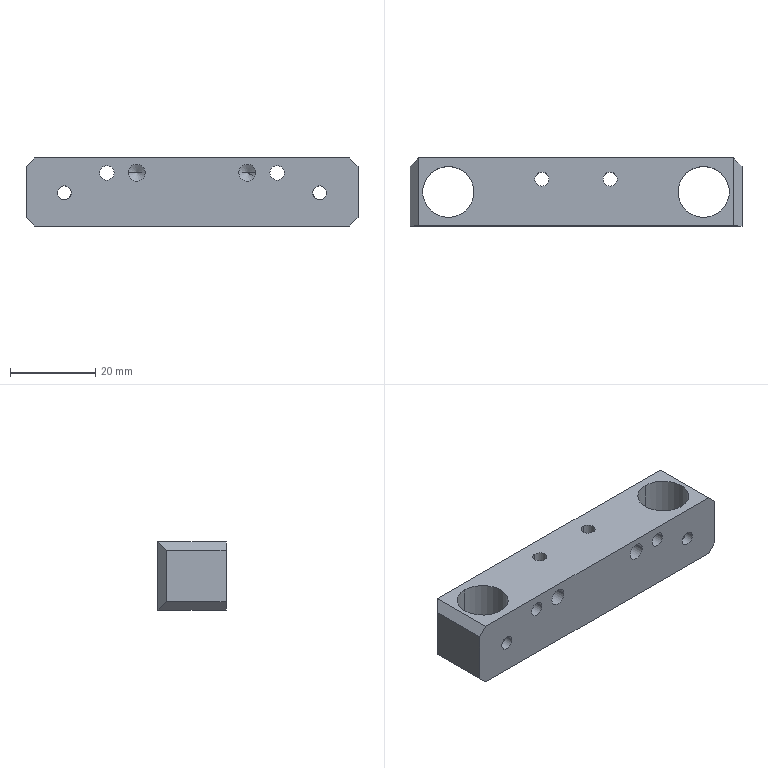NC program | NX | posted with a generic post | part box 78 x 16 x 16 mm
Lines 1 to 910 of 3743:
N10 G17 G21 G94 G90
(DRILLING , TOOL : ZXZ)
N12 T21 M6
N14 G54
N16 G17 G0 G90 X-30. Y0.2 B0. C0. S3500 M3
N18 G43 Z30. H21
N20 G94 G81 G98 Z-1. F250. R3.
N22 X-20. Y-4.5
N24 X-13.
N26 X13.
N28 X20.
N30 X30. Y0.2
N32 G80
N34 G0 X30. Y0.2 Z30.
N36 M5
(DRILLING_COPY_1 , TOOL : 3.4ZT)
N38 T24 M6
N40 G54
N42 G17 G0 G90 X-20. Y-4.5 B0. C0. S2000 M3
N44 G43 Z30. H24
N46 G94 G83 G98 Z-15.121 F150. Q2. R3.
N48 X-13. Z-11.021
N50 X13.
N52 X20. Z-15.121
N54 G80
N56 G0 X20. Y-4.5 Z30.
N58 M5
(DRILLING_COPY_1_COPY , TOOL : 3.3ZT)
N60 T13 M6
N62 G54
N64 G17 G0 G90 X-30. Y0.2 B0. C0. S2000 M3
N66 G43 Z30. H13
N68 G94 G83 G98 Z-17.991 F150. Q2. R3.
N70 X30.
N72 G80
N74 G0 X30. Y0.2 Z30.
N76 M5
(HOLE_MILLING_2 , TOOL : D2)
N78 T18 M6
N80 G54
N82 G17 G0 G90 X-13. Y-4.5 B0. C0. S7500 M3
N84 G43 Z30. H18
N86 Z0.5
N88 G94 G3 X-13.485 Y-4.015 R0.485 F800.
N90 X-13.97 Y-4.5 R0.485
N92 X-13.97 Y-4.5 Z0.475 I0.97 J0.
N94 X-13.97 Y-4.5 Z0.45 I0.97 J0.
N96 X-13.97 Y-4.5 Z0.425 I0.97 J0.
N98 X-13.97 Y-4.5 Z0.4 I0.97 J0.
N100 X-13.97 Y-4.5 Z0.375 I0.97 J0.
N102 X-13.97 Y-4.5 Z0.35 I0.97 J0.
N104 X-13.97 Y-4.5 Z0.325 I0.97 J0.
N106 X-13.97 Y-4.5 Z0.3 I0.97 J0.
N108 X-13.97 Y-4.5 Z0.275 I0.97 J0.
N110 X-13.97 Y-4.5 Z0.25 I0.97 J0.
N112 X-13.97 Y-4.5 Z0.225 I0.97 J0.
N114 X-13.97 Y-4.5 Z0.2 I0.97 J0.
N116 X-13.97 Y-4.5 Z0.175 I0.97 J0.
N118 X-13.97 Y-4.5 Z0.15 I0.97 J0.
N120 X-13.97 Y-4.5 Z0.125 I0.97 J0.
N122 X-13.97 Y-4.5 Z0.1 I0.97 J0.
N124 X-13.97 Y-4.5 Z0.075 I0.97 J0.
N126 X-13.97 Y-4.5 Z0.05 I0.97 J0.
N128 X-13.97 Y-4.5 Z0.025 I0.97 J0.
N130 X-13.97 Y-4.5 Z0. I0.97 J0.
N132 X-13.97 Y-4.5 Z-0.025 I0.97 J0.
N134 X-13.97 Y-4.5 Z-0.05 I0.97 J0.
N136 X-13.97 Y-4.5 Z-0.075 I0.97 J0.
N138 X-13.97 Y-4.5 Z-0.1 I0.97 J0.
N140 X-13.97 Y-4.5 Z-0.125 I0.97 J0.
N142 X-13.97 Y-4.5 Z-0.15 I0.97 J0.
N144 X-13.97 Y-4.5 Z-0.175 I0.97 J0.
N146 X-13.97 Y-4.5 Z-0.2 I0.97 J0.
N148 X-13.97 Y-4.5 Z-0.225 I0.97 J0.
N150 X-13.97 Y-4.5 Z-0.25 I0.97 J0.
N152 X-13.97 Y-4.5 Z-0.275 I0.97 J0.
N154 X-13.97 Y-4.5 Z-0.3 I0.97 J0.
N156 X-13.97 Y-4.5 Z-0.325 I0.97 J0.
N158 X-13.97 Y-4.5 Z-0.35 I0.97 J0.
N160 X-13.97 Y-4.5 Z-0.375 I0.97 J0.
N162 X-13.97 Y-4.5 Z-0.4 I0.97 J0.
N164 X-13.97 Y-4.5 Z-0.425 I0.97 J0.
N166 X-13.97 Y-4.5 Z-0.45 I0.97 J0.
N168 X-13.97 Y-4.5 Z-0.475 I0.97 J0.
N170 X-13.97 Y-4.5 Z-0.5 I0.97 J0.
N172 X-13.97 Y-4.5 Z-0.525 I0.97 J0.
N174 X-13.97 Y-4.5 Z-0.55 I0.97 J0.
N176 X-13.97 Y-4.5 Z-0.575 I0.97 J0.
N178 X-13.97 Y-4.5 Z-0.6 I0.97 J0.
N180 X-13.97 Y-4.5 Z-0.625 I0.97 J0.
N182 X-13.97 Y-4.5 Z-0.65 I0.97 J0.
N184 X-13.97 Y-4.5 Z-0.675 I0.97 J0.
N186 X-13.97 Y-4.5 Z-0.7 I0.97 J0.
N188 X-13.97 Y-4.5 Z-0.725 I0.97 J0.
N190 X-13.97 Y-4.5 Z-0.75 I0.97 J0.
N192 X-13.97 Y-4.5 Z-0.775 I0.97 J0.
N194 X-13.97 Y-4.5 Z-0.8 I0.97 J0.
N196 X-13.97 Y-4.5 Z-0.825 I0.97 J0.
N198 X-13.97 Y-4.5 Z-0.85 I0.97 J0.
N200 X-13.97 Y-4.5 Z-0.875 I0.97 J0.
N202 X-13.97 Y-4.5 Z-0.9 I0.97 J0.
N204 X-13.97 Y-4.5 Z-0.925 I0.97 J0.
N206 X-13.97 Y-4.5 Z-0.95 I0.97 J0.
N208 X-13.97 Y-4.5 Z-0.975 I0.97 J0.
N210 X-13.97 Y-4.5 Z-1. I0.97 J0.
N212 X-13.97 Y-4.5 Z-1.025 I0.97 J0.
N214 X-13.97 Y-4.5 Z-1.05 I0.97 J0.
N216 X-13.97 Y-4.5 Z-1.075 I0.97 J0.
N218 X-13.97 Y-4.5 Z-1.1 I0.97 J0.
N220 X-13.97 Y-4.5 Z-1.125 I0.97 J0.
N222 X-13.97 Y-4.5 Z-1.15 I0.97 J0.
N224 X-13.97 Y-4.5 Z-1.175 I0.97 J0.
N226 X-13.97 Y-4.5 Z-1.2 I0.97 J0.
N228 X-13.97 Y-4.5 Z-1.225 I0.97 J0.
N230 X-13.97 Y-4.5 Z-1.25 I0.97 J0.
N232 X-13.97 Y-4.5 Z-1.275 I0.97 J0.
N234 X-13.97 Y-4.5 Z-1.3 I0.97 J0.
N236 X-13.97 Y-4.5 Z-1.325 I0.97 J0.
N238 X-13.97 Y-4.5 Z-1.35 I0.97 J0.
N240 X-13.97 Y-4.5 Z-1.375 I0.97 J0.
N242 X-13.97 Y-4.5 Z-1.4 I0.97 J0.
N244 X-13.97 Y-4.5 Z-1.425 I0.97 J0.
N246 X-13.97 Y-4.5 Z-1.45 I0.97 J0.
N248 X-13.97 Y-4.5 Z-1.475 I0.97 J0.
N250 X-13.97 Y-4.5 Z-1.5 I0.97 J0.
N252 X-13.97 Y-4.5 Z-1.525 I0.97 J0.
N254 X-13.97 Y-4.5 Z-1.55 I0.97 J0.
N256 X-13.97 Y-4.5 Z-1.575 I0.97 J0.
N258 X-13.97 Y-4.5 Z-1.6 I0.97 J0.
N260 X-13.97 Y-4.5 Z-1.625 I0.97 J0.
N262 X-13.97 Y-4.5 Z-1.65 I0.97 J0.
N264 X-13.97 Y-4.5 Z-1.675 I0.97 J0.
N266 X-13.97 Y-4.5 Z-1.7 I0.97 J0.
N268 X-13.97 Y-4.5 Z-1.725 I0.97 J0.
N270 X-13.97 Y-4.5 Z-1.75 I0.97 J0.
N272 X-13.97 Y-4.5 Z-1.775 I0.97 J0.
N274 X-13.97 Y-4.5 Z-1.8 I0.97 J0.
N276 X-13.97 Y-4.5 Z-1.825 I0.97 J0.
N278 X-13.97 Y-4.5 Z-1.85 I0.97 J0.
N280 X-13.97 Y-4.5 Z-1.875 I0.97 J0.
N282 X-13.97 Y-4.5 Z-1.9 I0.97 J0.
N284 X-13.97 Y-4.5 Z-1.925 I0.97 J0.
N286 X-13.97 Y-4.5 Z-1.95 I0.97 J0.
N288 X-13.97 Y-4.5 Z-1.975 I0.97 J0.
N290 X-13.97 Y-4.5 Z-2. I0.97 J0.
N292 X-13.97 Y-4.5 Z-2.025 I0.97 J0.
N294 X-13.97 Y-4.5 Z-2.05 I0.97 J0.
N296 X-13.97 Y-4.5 Z-2.075 I0.97 J0.
N298 X-13.97 Y-4.5 Z-2.1 I0.97 J0.
N300 X-13.97 Y-4.5 Z-2.125 I0.97 J0.
N302 X-13.97 Y-4.5 Z-2.15 I0.97 J0.
N304 X-13.97 Y-4.5 Z-2.175 I0.97 J0.
N306 X-13.97 Y-4.5 Z-2.2 I0.97 J0.
N308 X-13.97 Y-4.5 Z-2.225 I0.97 J0.
N310 X-13.97 Y-4.5 Z-2.25 I0.97 J0.
N312 X-13.97 Y-4.5 Z-2.275 I0.97 J0.
N314 X-13.97 Y-4.5 Z-2.3 I0.97 J0.
N316 X-13.97 Y-4.5 Z-2.325 I0.97 J0.
N318 X-13.97 Y-4.5 Z-2.35 I0.97 J0.
N320 X-13.97 Y-4.5 Z-2.375 I0.97 J0.
N322 X-13.97 Y-4.5 Z-2.4 I0.97 J0.
N324 X-13.97 Y-4.5 Z-2.425 I0.97 J0.
N326 X-13.97 Y-4.5 Z-2.45 I0.97 J0.
N328 X-13.97 Y-4.5 Z-2.475 I0.97 J0.
N330 X-13.97 Y-4.5 Z-2.5 I0.97 J0.
N332 X-13.97 Y-4.5 Z-2.525 I0.97 J0.
N334 X-13.97 Y-4.5 Z-2.55 I0.97 J0.
N336 X-13.97 Y-4.5 Z-2.575 I0.97 J0.
N338 X-13.97 Y-4.5 Z-2.6 I0.97 J0.
N340 X-13.97 Y-4.5 Z-2.625 I0.97 J0.
N342 X-13.97 Y-4.5 Z-2.65 I0.97 J0.
N344 X-13.97 Y-4.5 Z-2.675 I0.97 J0.
N346 X-13.97 Y-4.5 Z-2.7 I0.97 J0.
N348 X-13.97 Y-4.5 Z-2.725 I0.97 J0.
N350 X-13.97 Y-4.5 Z-2.75 I0.97 J0.
N352 X-13.97 Y-4.5 Z-2.775 I0.97 J0.
N354 X-13.97 Y-4.5 Z-2.8 I0.97 J0.
N356 X-13.97 Y-4.5 Z-2.825 I0.97 J0.
N358 X-13.97 Y-4.5 Z-2.85 I0.97 J0.
N360 X-13.97 Y-4.5 Z-2.875 I0.97 J0.
N362 X-13.97 Y-4.5 Z-2.9 I0.97 J0.
N364 X-13.97 Y-4.5 Z-2.925 I0.97 J0.
N366 X-13.97 Y-4.5 Z-2.95 I0.97 J0.
N368 X-13.97 Y-4.5 Z-2.975 I0.97 J0.
N370 X-13.97 Y-4.5 Z-3. I0.97 J0.
N372 X-13.97 Y-4.5 Z-3.025 I0.97 J0.
N374 X-13.97 Y-4.5 Z-3.05 I0.97 J0.
N376 X-13.97 Y-4.5 Z-3.075 I0.97 J0.
N378 X-13.97 Y-4.5 Z-3.1 I0.97 J0.
N380 X-13.97 Y-4.5 Z-3.125 I0.97 J0.
N382 X-13.97 Y-4.5 Z-3.15 I0.97 J0.
N384 X-13.97 Y-4.5 Z-3.175 I0.97 J0.
N386 X-13.97 Y-4.5 Z-3.2 I0.97 J0.
N388 X-13.97 Y-4.5 Z-3.225 I0.97 J0.
N390 X-13.97 Y-4.5 Z-3.25 I0.97 J0.
N392 X-13.97 Y-4.5 Z-3.275 I0.97 J0.
N394 X-13.97 Y-4.5 Z-3.3 I0.97 J0.
N396 X-13.97 Y-4.5 Z-3.325 I0.97 J0.
N398 X-13.97 Y-4.5 Z-3.35 I0.97 J0.
N400 X-13.97 Y-4.5 Z-3.375 I0.97 J0.
N402 X-13.97 Y-4.5 Z-3.4 I0.97 J0.
N404 X-13.97 Y-4.5 Z-3.425 I0.97 J0.
N406 X-13.97 Y-4.5 Z-3.45 I0.97 J0.
N408 X-13.97 Y-4.5 Z-3.475 I0.97 J0.
N410 X-13.97 Y-4.5 Z-3.5 I0.97 J0.
N412 X-13.97 Y-4.5 Z-3.525 I0.97 J0.
N414 X-13.97 Y-4.5 Z-3.55 I0.97 J0.
N416 X-13.97 Y-4.5 Z-3.575 I0.97 J0.
N418 X-13.97 Y-4.5 Z-3.6 I0.97 J0.
N420 X-13.97 Y-4.5 Z-3.625 I0.97 J0.
N422 X-13.97 Y-4.5 Z-3.65 I0.97 J0.
N424 X-13.97 Y-4.5 Z-3.675 I0.97 J0.
N426 X-13.97 Y-4.5 Z-3.7 I0.97 J0.
N428 X-13.97 Y-4.5 Z-3.725 I0.97 J0.
N430 X-13.97 Y-4.5 Z-3.75 I0.97 J0.
N432 X-13.97 Y-4.5 Z-3.775 I0.97 J0.
N434 X-13.97 Y-4.5 Z-3.8 I0.97 J0.
N436 X-13.97 Y-4.5 Z-3.825 I0.97 J0.
N438 X-13.97 Y-4.5 Z-3.85 I0.97 J0.
N440 X-13.97 Y-4.5 Z-3.875 I0.97 J0.
N442 X-13.97 Y-4.5 Z-3.9 I0.97 J0.
N444 X-13.97 Y-4.5 Z-3.925 I0.97 J0.
N446 X-13.97 Y-4.5 Z-3.95 I0.97 J0.
N448 X-13.97 Y-4.5 Z-3.975 I0.97 J0.
N450 X-13.97 Y-4.5 Z-4. I0.97 J0.
N452 X-13.97 Y-4.5 Z-4.025 I0.97 J0.
N454 X-13.97 Y-4.5 Z-4.05 I0.97 J0.
N456 X-13.97 Y-4.5 Z-4.075 I0.97 J0.
N458 X-13.97 Y-4.5 Z-4.1 I0.97 J0.
N460 X-13.97 Y-4.5 Z-4.125 I0.97 J0.
N462 X-13.97 Y-4.5 Z-4.15 I0.97 J0.
N464 X-13.97 Y-4.5 Z-4.175 I0.97 J0.
N466 X-13.97 Y-4.5 Z-4.2 I0.97 J0.
N468 X-13.97 Y-4.5 Z-4.225 I0.97 J0.
N470 X-13.97 Y-4.5 Z-4.25 I0.97 J0.
N472 X-13.97 Y-4.5 Z-4.275 I0.97 J0.
N474 X-13.97 Y-4.5 Z-4.3 I0.97 J0.
N476 X-13.97 Y-4.5 Z-4.325 I0.97 J0.
N478 X-13.97 Y-4.5 Z-4.35 I0.97 J0.
N480 X-13.97 Y-4.5 Z-4.375 I0.97 J0.
N482 X-13.97 Y-4.5 Z-4.4 I0.97 J0.
N484 X-13.97 Y-4.5 Z-4.425 I0.97 J0.
N486 X-13.97 Y-4.5 Z-4.45 I0.97 J0.
N488 X-13.97 Y-4.5 Z-4.475 I0.97 J0.
N490 X-13.97 Y-4.5 Z-4.5 I0.97 J0.
N492 X-13.97 Y-4.5 Z-4.525 I0.97 J0.
N494 X-13.97 Y-4.5 Z-4.55 I0.97 J0.
N496 X-13.97 Y-4.5 Z-4.575 I0.97 J0.
N498 X-13.97 Y-4.5 Z-4.6 I0.97 J0.
N500 X-13.97 Y-4.5 Z-4.625 I0.97 J0.
N502 X-13.97 Y-4.5 Z-4.65 I0.97 J0.
N504 X-13.97 Y-4.5 Z-4.675 I0.97 J0.
N506 X-13.97 Y-4.5 Z-4.7 I0.97 J0.
N508 X-13.97 Y-4.5 Z-4.725 I0.97 J0.
N510 X-13.97 Y-4.5 Z-4.75 I0.97 J0.
N512 X-13.97 Y-4.5 Z-4.775 I0.97 J0.
N514 X-13.97 Y-4.5 Z-4.8 I0.97 J0.
N516 X-13.97 Y-4.5 Z-4.825 I0.97 J0.
N518 X-13.97 Y-4.5 Z-4.85 I0.97 J0.
N520 X-13.97 Y-4.5 Z-4.875 I0.97 J0.
N522 X-13.97 Y-4.5 Z-4.9 I0.97 J0.
N524 X-13.97 Y-4.5 Z-4.925 I0.97 J0.
N526 X-13.97 Y-4.5 Z-4.95 I0.97 J0.
N528 X-13.97 Y-4.5 Z-4.975 I0.97 J0.
N530 X-13.97 Y-4.5 Z-5. I0.97 J0.
N532 X-13.97 Y-4.5 Z-5.025 I0.97 J0.
N534 X-13.97 Y-4.5 Z-5.05 I0.97 J0.
N536 X-13.97 Y-4.5 Z-5.075 I0.97 J0.
N538 X-13.97 Y-4.5 Z-5.1 I0.97 J0.
N540 X-13.97 Y-4.5 Z-5.125 I0.97 J0.
N542 X-13.97 Y-4.5 Z-5.15 I0.97 J0.
N544 X-13.97 Y-4.5 Z-5.175 I0.97 J0.
N546 X-13.97 Y-4.5 Z-5.2 I0.97 J0.
N548 X-13.97 Y-4.5 Z-5.225 I0.97 J0.
N550 X-13.97 Y-4.5 Z-5.25 I0.97 J0.
N552 X-13.97 Y-4.5 Z-5.275 I0.97 J0.
N554 X-13.97 Y-4.5 Z-5.3 I0.97 J0.
N556 X-13.97 Y-4.5 Z-5.325 I0.97 J0.
N558 X-13.97 Y-4.5 Z-5.35 I0.97 J0.
N560 X-13.97 Y-4.5 Z-5.375 I0.97 J0.
N562 X-13.97 Y-4.5 Z-5.4 I0.97 J0.
N564 X-13.97 Y-4.5 Z-5.425 I0.97 J0.
N566 X-13.97 Y-4.5 Z-5.45 I0.97 J0.
N568 X-13.97 Y-4.5 Z-5.475 I0.97 J0.
N570 X-13.97 Y-4.5 Z-5.5 I0.97 J0.
N572 X-13.97 Y-4.5 Z-5.525 I0.97 J0.
N574 X-13.97 Y-4.5 Z-5.55 I0.97 J0.
N576 X-13.97 Y-4.5 Z-5.575 I0.97 J0.
N578 X-13.97 Y-4.5 Z-5.6 I0.97 J0.
N580 X-13.97 Y-4.5 Z-5.625 I0.97 J0.
N582 X-13.97 Y-4.5 Z-5.65 I0.97 J0.
N584 X-13.97 Y-4.5 Z-5.675 I0.97 J0.
N586 X-13.97 Y-4.5 Z-5.7 I0.97 J0.
N588 X-13.97 Y-4.5 Z-5.725 I0.97 J0.
N590 X-13.97 Y-4.5 Z-5.75 I0.97 J0.
N592 X-13.97 Y-4.5 Z-5.775 I0.97 J0.
N594 X-13.97 Y-4.5 Z-5.8 I0.97 J0.
N596 X-13.97 Y-4.5 Z-5.825 I0.97 J0.
N598 X-13.97 Y-4.5 Z-5.85 I0.97 J0.
N600 X-13.97 Y-4.5 Z-5.875 I0.97 J0.
N602 X-13.97 Y-4.5 Z-5.9 I0.97 J0.
N604 X-13.97 Y-4.5 Z-5.925 I0.97 J0.
N606 X-13.97 Y-4.5 Z-5.95 I0.97 J0.
N608 X-13.97 Y-4.5 Z-5.975 I0.97 J0.
N610 X-13.97 Y-4.5 Z-6. I0.97 J0.
N612 X-13.97 Y-4.5 Z-6.025 I0.97 J0.
N614 X-13.97 Y-4.5 Z-6.05 I0.97 J0.
N616 X-13.97 Y-4.5 Z-6.075 I0.97 J0.
N618 X-13.97 Y-4.5 Z-6.1 I0.97 J0.
N620 X-13.97 Y-4.5 Z-6.125 I0.97 J0.
N622 X-13.97 Y-4.5 Z-6.15 I0.97 J0.
N624 X-13.97 Y-4.5 Z-6.175 I0.97 J0.
N626 X-13.97 Y-4.5 Z-6.2 I0.97 J0.
N628 X-13.97 Y-4.5 Z-6.225 I0.97 J0.
N630 X-13.97 Y-4.5 Z-6.25 I0.97 J0.
N632 X-13.97 Y-4.5 Z-6.275 I0.97 J0.
N634 X-13.97 Y-4.5 Z-6.3 I0.97 J0.
N636 X-13.97 Y-4.5 Z-6.325 I0.97 J0.
N638 X-13.97 Y-4.5 Z-6.35 I0.97 J0.
N640 X-13.97 Y-4.5 Z-6.375 I0.97 J0.
N642 X-13.97 Y-4.5 Z-6.4 I0.97 J0.
N644 X-13.97 Y-4.5 Z-6.425 I0.97 J0.
N646 X-13.97 Y-4.5 Z-6.45 I0.97 J0.
N648 X-13.97 Y-4.5 Z-6.475 I0.97 J0.
N650 X-13.97 Y-4.5 Z-6.5 I0.97 J0.
N652 X-13.97 Y-4.5 Z-6.525 I0.97 J0.
N654 X-13.97 Y-4.5 Z-6.55 I0.97 J0.
N656 X-13.97 Y-4.5 Z-6.575 I0.97 J0.
N658 X-13.97 Y-4.5 Z-6.6 I0.97 J0.
N660 X-13.97 Y-4.5 Z-6.625 I0.97 J0.
N662 X-13.97 Y-4.5 Z-6.65 I0.97 J0.
N664 X-13.97 Y-4.5 Z-6.675 I0.97 J0.
N666 X-13.97 Y-4.5 Z-6.7 I0.97 J0.
N668 X-13.97 Y-4.5 Z-6.725 I0.97 J0.
N670 X-13.97 Y-4.5 Z-6.75 I0.97 J0.
N672 X-13.97 Y-4.5 Z-6.775 I0.97 J0.
N674 X-13.97 Y-4.5 Z-6.8 I0.97 J0.
N676 X-13.97 Y-4.5 Z-6.825 I0.97 J0.
N678 X-13.97 Y-4.5 Z-6.85 I0.97 J0.
N680 X-13.97 Y-4.5 Z-6.875 I0.97 J0.
N682 X-13.97 Y-4.5 Z-6.9 I0.97 J0.
N684 X-13.97 Y-4.5 Z-6.925 I0.97 J0.
N686 X-13.97 Y-4.5 Z-6.95 I0.97 J0.
N688 X-13.97 Y-4.5 Z-6.975 I0.97 J0.
N690 X-13.97 Y-4.5 Z-7. I0.97 J0.
N692 X-13.97 Y-4.5 Z-7.025 I0.97 J0.
N694 X-13.97 Y-4.5 Z-7.05 I0.97 J0.
N696 X-13.97 Y-4.5 Z-7.075 I0.97 J0.
N698 X-13.97 Y-4.5 Z-7.1 I0.97 J0.
N700 X-13.97 Y-4.5 Z-7.125 I0.97 J0.
N702 X-13.97 Y-4.5 Z-7.15 I0.97 J0.
N704 X-13.97 Y-4.5 Z-7.175 I0.97 J0.
N706 X-13.97 Y-4.5 Z-7.2 I0.97 J0.
N708 X-13.97 Y-4.5 Z-7.225 I0.97 J0.
N710 X-13.97 Y-4.5 Z-7.25 I0.97 J0.
N712 X-13.97 Y-4.5 Z-7.275 I0.97 J0.
N714 X-13.97 Y-4.5 Z-7.3 I0.97 J0.
N716 X-13.97 Y-4.5 Z-7.325 I0.97 J0.
N718 X-13.97 Y-4.5 Z-7.35 I0.97 J0.
N720 X-13.97 Y-4.5 Z-7.375 I0.97 J0.
N722 X-13.97 Y-4.5 Z-7.4 I0.97 J0.
N724 X-13.97 Y-4.5 Z-7.425 I0.97 J0.
N726 X-13.97 Y-4.5 Z-7.45 I0.97 J0.
N728 X-13.97 Y-4.5 Z-7.475 I0.97 J0.
N730 X-13.97 Y-4.5 Z-7.5 I0.97 J0.
N732 X-13.97 Y-4.5 Z-7.525 I0.97 J0.
N734 X-13.97 Y-4.5 Z-7.55 I0.97 J0.
N736 X-13.97 Y-4.5 Z-7.575 I0.97 J0.
N738 X-13.97 Y-4.5 Z-7.6 I0.97 J0.
N740 X-13.97 Y-4.5 Z-7.625 I0.97 J0.
N742 X-13.97 Y-4.5 Z-7.65 I0.97 J0.
N744 X-13.97 Y-4.5 Z-7.675 I0.97 J0.
N746 X-13.97 Y-4.5 Z-7.7 I0.97 J0.
N748 X-13.97 Y-4.5 Z-7.725 I0.97 J0.
N750 X-13.97 Y-4.5 Z-7.75 I0.97 J0.
N752 X-13.97 Y-4.5 Z-7.775 I0.97 J0.
N754 X-13.97 Y-4.5 Z-7.8 I0.97 J0.
N756 X-13.97 Y-4.5 Z-7.825 I0.97 J0.
N758 X-13.97 Y-4.5 Z-7.85 I0.97 J0.
N760 X-13.97 Y-4.5 Z-7.875 I0.97 J0.
N762 X-13.97 Y-4.5 Z-7.9 I0.97 J0.
N764 X-13.97 Y-4.5 Z-7.925 I0.97 J0.
N766 X-13.97 Y-4.5 Z-7.95 I0.97 J0.
N768 X-13.97 Y-4.5 Z-7.975 I0.97 J0.
N770 X-13.97 Y-4.5 Z-8. I0.97 J0.
N772 X-13.97 Y-4.5 Z-8.025 I0.97 J0.
N774 X-13.97 Y-4.5 Z-8.05 I0.97 J0.
N776 X-13.97 Y-4.5 Z-8.075 I0.97 J0.
N778 X-13.97 Y-4.5 Z-8.1 I0.97 J0.
N780 X-13.97 Y-4.5 Z-8.125 I0.97 J0.
N782 X-13.97 Y-4.5 Z-8.15 I0.97 J0.
N784 X-13.97 Y-4.5 Z-8.175 I0.97 J0.
N786 X-13.97 Y-4.5 Z-8.2 I0.97 J0.
N788 X-13.97 Y-4.5 Z-8.225 I0.97 J0.
N790 X-13.97 Y-4.5 Z-8.25 I0.97 J0.
N792 X-13.97 Y-4.5 Z-8.275 I0.97 J0.
N794 X-13.97 Y-4.5 Z-8.3 I0.97 J0.
N796 X-13.97 Y-4.5 Z-8.325 I0.97 J0.
N798 X-13.97 Y-4.5 Z-8.35 I0.97 J0.
N800 X-13.97 Y-4.5 Z-8.375 I0.97 J0.
N802 X-13.97 Y-4.5 Z-8.4 I0.97 J0.
N804 X-13.97 Y-4.5 Z-8.425 I0.97 J0.
N806 X-13.97 Y-4.5 Z-8.45 I0.97 J0.
N808 X-13.97 Y-4.5 Z-8.475 I0.97 J0.
N810 X-13.97 Y-4.5 Z-8.5 I0.97 J0.
N812 X-13.97 Y-4.5 Z-8.525 I0.97 J0.
N814 X-13.97 Y-4.5 Z-8.55 I0.97 J0.
N816 X-13.97 Y-4.5 Z-8.575 I0.97 J0.
N818 X-13.97 Y-4.5 Z-8.6 I0.97 J0.
N820 X-13.97 Y-4.5 Z-8.625 I0.97 J0.
N822 X-13.97 Y-4.5 Z-8.65 I0.97 J0.
N824 X-13.97 Y-4.5 Z-8.675 I0.97 J0.
N826 X-13.97 Y-4.5 Z-8.7 I0.97 J0.
N828 X-13.97 Y-4.5 Z-8.725 I0.97 J0.
N830 X-13.97 Y-4.5 Z-8.75 I0.97 J0.
N832 X-13.97 Y-4.5 Z-8.775 I0.97 J0.
N834 X-13.97 Y-4.5 Z-8.8 I0.97 J0.
N836 X-13.97 Y-4.5 Z-8.825 I0.97 J0.
N838 X-13.97 Y-4.5 Z-8.85 I0.97 J0.
N840 X-13.97 Y-4.5 Z-8.875 I0.97 J0.
N842 X-13.97 Y-4.5 Z-8.9 I0.97 J0.
N844 X-13.97 Y-4.5 Z-8.925 I0.97 J0.
N846 X-13.97 Y-4.5 Z-8.95 I0.97 J0.
N848 X-13.97 Y-4.5 Z-8.975 I0.97 J0.
N850 X-13.97 Y-4.5 Z-9. I0.97 J0.
N852 X-13.97 Y-4.5 Z-9.025 I0.97 J0.
N854 X-13.97 Y-4.5 Z-9.05 I0.97 J0.
N856 X-13.97 Y-4.5 Z-9.075 I0.97 J0.
N858 X-13.97 Y-4.5 Z-9.1 I0.97 J0.
N860 X-13.97 Y-4.5 Z-9.125 I0.97 J0.
N862 X-13.97 Y-4.5 Z-9.15 I0.97 J0.
N864 X-13.97 Y-4.5 Z-9.175 I0.97 J0.
N866 X-13.97 Y-4.5 Z-9.2 I0.97 J0.
N868 X-13.97 Y-4.5 Z-9.225 I0.97 J0.
N870 X-13.97 Y-4.5 Z-9.25 I0.97 J0.
N872 X-13.97 Y-4.5 Z-9.275 I0.97 J0.
N874 X-13.97 Y-4.5 Z-9.3 I0.97 J0.
N876 X-13.97 Y-4.5 Z-9.325 I0.97 J0.
N878 X-13.97 Y-4.5 Z-9.35 I0.97 J0.
N880 X-13.97 Y-4.5 Z-9.375 I0.97 J0.
N882 X-13.97 Y-4.5 Z-9.4 I0.97 J0.
N884 X-13.97 Y-4.5 Z-9.425 I0.97 J0.
N886 X-13.97 Y-4.5 Z-9.45 I0.97 J0.
N888 X-13.97 Y-4.5 Z-9.475 I0.97 J0.
N890 X-13.97 Y-4.5 Z-9.5 I0.97 J0.
N892 X-13.97 Y-4.5 Z-9.525 I0.97 J0.
N894 X-13.97 Y-4.5 Z-9.55 I0.97 J0.
N896 X-13.97 Y-4.5 Z-9.575 I0.97 J0.
N898 X-13.97 Y-4.5 Z-9.6 I0.97 J0.
N900 X-13.97 Y-4.5 Z-9.625 I0.97 J0.
N902 X-13.97 Y-4.5 Z-9.65 I0.97 J0.
N904 X-13.97 Y-4.5 Z-9.675 I0.97 J0.
N906 X-13.97 Y-4.5 Z-9.7 I0.97 J0.
N908 X-13.97 Y-4.5 Z-9.725 I0.97 J0.
N910 X-13.97 Y-4.5 Z-9.75 I0.97 J0.
N912 X-13.97 Y-4.5 Z-9.775 I0.97 J0.
N914 X-13.97 Y-4.5 Z-9.8 I0.97 J0.
N916 X-13.97 Y-4.5 Z-9.825 I0.97 J0.
N918 X-13.97 Y-4.5 Z-9.85 I0.97 J0.
N920 X-13.97 Y-4.5 Z-9.875 I0.97 J0.
N922 X-13.97 Y-4.5 Z-9.9 I0.97 J0.
N924 X-13.97 Y-4.5 Z-9.925 I0.97 J0.
N926 X-13.97 Y-4.5 Z-9.95 I0.97 J0.
N928 X-13.97 Y-4.5 Z-9.975 I0.97 J0.
N930 X-13.97 Y-4.5 Z-10. I0.97 J0.
N932 X-13. Y-5.47 R0.97
N934 X-13.97 Y-4.5 R-0.97
N936 X-13.485 Y-4.985 R0.485
N938 X-13. Y-4.5 R0.485
N940 G0 Z30.
N942 X13.
N944 Z0.5
N946 G3 X12.515 Y-4.015 R0.485
N948 X12.03 Y-4.5 R0.485
N950 X12.03 Y-4.5 Z0.475 I0.97 J0.
N952 X12.03 Y-4.5 Z0.45 I0.97 J0.
N954 X12.03 Y-4.5 Z0.425 I0.97 J0.
N956 X12.03 Y-4.5 Z0.4 I0.97 J0.
N958 X12.03 Y-4.5 Z0.375 I0.97 J0.
N960 X12.03 Y-4.5 Z0.35 I0.97 J0.
N962 X12.03 Y-4.5 Z0.325 I0.97 J0.
N964 X12.03 Y-4.5 Z0.3 I0.97 J0.
N966 X12.03 Y-4.5 Z0.275 I0.97 J0.
N968 X12.03 Y-4.5 Z0.25 I0.97 J0.
N970 X12.03 Y-4.5 Z0.225 I0.97 J0.
N972 X12.03 Y-4.5 Z0.2 I0.97 J0.
N974 X12.03 Y-4.5 Z0.175 I0.97 J0.
N976 X12.03 Y-4.5 Z0.15 I0.97 J0.
N978 X12.03 Y-4.5 Z0.125 I0.97 J0.
N980 X12.03 Y-4.5 Z0.1 I0.97 J0.
N982 X12.03 Y-4.5 Z0.075 I0.97 J0.
N984 X12.03 Y-4.5 Z0.05 I0.97 J0.
N986 X12.03 Y-4.5 Z0.025 I0.97 J0.
N988 X12.03 Y-4.5 Z0. I0.97 J0.
N990 X12.03 Y-4.5 Z-0.025 I0.97 J0.
N992 X12.03 Y-4.5 Z-0.05 I0.97 J0.
N994 X12.03 Y-4.5 Z-0.075 I0.97 J0.
N996 X12.03 Y-4.5 Z-0.1 I0.97 J0.
N998 X12.03 Y-4.5 Z-0.125 I0.97 J0.
N1000 X12.03 Y-4.5 Z-0.15 I0.97 J0.
N1002 X12.03 Y-4.5 Z-0.175 I0.97 J0.
N1004 X12.03 Y-4.5 Z-0.2 I0.97 J0.
N1006 X12.03 Y-4.5 Z-0.225 I0.97 J0.
N1008 X12.03 Y-4.5 Z-0.25 I0.97 J0.
N1010 X12.03 Y-4.5 Z-0.275 I0.97 J0.
N1012 X12.03 Y-4.5 Z-0.3 I0.97 J0.
N1014 X12.03 Y-4.5 Z-0.325 I0.97 J0.
N1016 X12.03 Y-4.5 Z-0.35 I0.97 J0.
N1018 X12.03 Y-4.5 Z-0.375 I0.97 J0.
N1020 X12.03 Y-4.5 Z-0.4 I0.97 J0.
N1022 X12.03 Y-4.5 Z-0.425 I0.97 J0.
N1024 X12.03 Y-4.5 Z-0.45 I0.97 J0.
N1026 X12.03 Y-4.5 Z-0.475 I0.97 J0.
N1028 X12.03 Y-4.5 Z-0.5 I0.97 J0.
N1030 X12.03 Y-4.5 Z-0.525 I0.97 J0.
N1032 X12.03 Y-4.5 Z-0.55 I0.97 J0.
N1034 X12.03 Y-4.5 Z-0.575 I0.97 J0.
N1036 X12.03 Y-4.5 Z-0.6 I0.97 J0.
N1038 X12.03 Y-4.5 Z-0.625 I0.97 J0.
N1040 X12.03 Y-4.5 Z-0.65 I0.97 J0.
N1042 X12.03 Y-4.5 Z-0.675 I0.97 J0.
N1044 X12.03 Y-4.5 Z-0.7 I0.97 J0.
N1046 X12.03 Y-4.5 Z-0.725 I0.97 J0.
N1048 X12.03 Y-4.5 Z-0.75 I0.97 J0.
N1050 X12.03 Y-4.5 Z-0.775 I0.97 J0.
N1052 X12.03 Y-4.5 Z-0.8 I0.97 J0.
N1054 X12.03 Y-4.5 Z-0.825 I0.97 J0.
N1056 X12.03 Y-4.5 Z-0.85 I0.97 J0.
N1058 X12.03 Y-4.5 Z-0.875 I0.97 J0.
N1060 X12.03 Y-4.5 Z-0.9 I0.97 J0.
N1062 X12.03 Y-4.5 Z-0.925 I0.97 J0.
N1064 X12.03 Y-4.5 Z-0.95 I0.97 J0.
N1066 X12.03 Y-4.5 Z-0.975 I0.97 J0.
N1068 X12.03 Y-4.5 Z-1. I0.97 J0.
N1070 X12.03 Y-4.5 Z-1.025 I0.97 J0.
N1072 X12.03 Y-4.5 Z-1.05 I0.97 J0.
N1074 X12.03 Y-4.5 Z-1.075 I0.97 J0.
N1076 X12.03 Y-4.5 Z-1.1 I0.97 J0.
N1078 X12.03 Y-4.5 Z-1.125 I0.97 J0.
N1080 X12.03 Y-4.5 Z-1.15 I0.97 J0.
N1082 X12.03 Y-4.5 Z-1.175 I0.97 J0.
N1084 X12.03 Y-4.5 Z-1.2 I0.97 J0.
N1086 X12.03 Y-4.5 Z-1.225 I0.97 J0.
N1088 X12.03 Y-4.5 Z-1.25 I0.97 J0.
N1090 X12.03 Y-4.5 Z-1.275 I0.97 J0.
N1092 X12.03 Y-4.5 Z-1.3 I0.97 J0.
N1094 X12.03 Y-4.5 Z-1.325 I0.97 J0.
N1096 X12.03 Y-4.5 Z-1.35 I0.97 J0.
N1098 X12.03 Y-4.5 Z-1.375 I0.97 J0.
N1100 X12.03 Y-4.5 Z-1.4 I0.97 J0.
N1102 X12.03 Y-4.5 Z-1.425 I0.97 J0.
N1104 X12.03 Y-4.5 Z-1.45 I0.97 J0.
N1106 X12.03 Y-4.5 Z-1.475 I0.97 J0.
N1108 X12.03 Y-4.5 Z-1.5 I0.97 J0.
N1110 X12.03 Y-4.5 Z-1.525 I0.97 J0.
N1112 X12.03 Y-4.5 Z-1.55 I0.97 J0.
N1114 X12.03 Y-4.5 Z-1.575 I0.97 J0.
N1116 X12.03 Y-4.5 Z-1.6 I0.97 J0.
N1118 X12.03 Y-4.5 Z-1.625 I0.97 J0.
N1120 X12.03 Y-4.5 Z-1.65 I0.97 J0.
N1122 X12.03 Y-4.5 Z-1.675 I0.97 J0.
N1124 X12.03 Y-4.5 Z-1.7 I0.97 J0.
N1126 X12.03 Y-4.5 Z-1.725 I0.97 J0.
N1128 X12.03 Y-4.5 Z-1.75 I0.97 J0.
N1130 X12.03 Y-4.5 Z-1.775 I0.97 J0.
N1132 X12.03 Y-4.5 Z-1.8 I0.97 J0.
N1134 X12.03 Y-4.5 Z-1.825 I0.97 J0.
N1136 X12.03 Y-4.5 Z-1.85 I0.97 J0.
N1138 X12.03 Y-4.5 Z-1.875 I0.97 J0.
N1140 X12.03 Y-4.5 Z-1.9 I0.97 J0.
N1142 X12.03 Y-4.5 Z-1.925 I0.97 J0.
N1144 X12.03 Y-4.5 Z-1.95 I0.97 J0.
N1146 X12.03 Y-4.5 Z-1.975 I0.97 J0.
N1148 X12.03 Y-4.5 Z-2. I0.97 J0.
N1150 X12.03 Y-4.5 Z-2.025 I0.97 J0.
N1152 X12.03 Y-4.5 Z-2.05 I0.97 J0.
N1154 X12.03 Y-4.5 Z-2.075 I0.97 J0.
N1156 X12.03 Y-4.5 Z-2.1 I0.97 J0.
N1158 X12.03 Y-4.5 Z-2.125 I0.97 J0.
N1160 X12.03 Y-4.5 Z-2.15 I0.97 J0.
N1162 X12.03 Y-4.5 Z-2.175 I0.97 J0.
N1164 X12.03 Y-4.5 Z-2.2 I0.97 J0.
N1166 X12.03 Y-4.5 Z-2.225 I0.97 J0.
N1168 X12.03 Y-4.5 Z-2.25 I0.97 J0.
N1170 X12.03 Y-4.5 Z-2.275 I0.97 J0.
N1172 X12.03 Y-4.5 Z-2.3 I0.97 J0.
N1174 X12.03 Y-4.5 Z-2.325 I0.97 J0.
N1176 X12.03 Y-4.5 Z-2.35 I0.97 J0.
N1178 X12.03 Y-4.5 Z-2.375 I0.97 J0.
N1180 X12.03 Y-4.5 Z-2.4 I0.97 J0.
N1182 X12.03 Y-4.5 Z-2.425 I0.97 J0.
N1184 X12.03 Y-4.5 Z-2.45 I0.97 J0.
N1186 X12.03 Y-4.5 Z-2.475 I0.97 J0.
N1188 X12.03 Y-4.5 Z-2.5 I0.97 J0.
N1190 X12.03 Y-4.5 Z-2.525 I0.97 J0.
N1192 X12.03 Y-4.5 Z-2.55 I0.97 J0.
N1194 X12.03 Y-4.5 Z-2.575 I0.97 J0.
N1196 X12.03 Y-4.5 Z-2.6 I0.97 J0.
N1198 X12.03 Y-4.5 Z-2.625 I0.97 J0.
N1200 X12.03 Y-4.5 Z-2.65 I0.97 J0.
N1202 X12.03 Y-4.5 Z-2.675 I0.97 J0.
N1204 X12.03 Y-4.5 Z-2.7 I0.97 J0.
N1206 X12.03 Y-4.5 Z-2.725 I0.97 J0.
N1208 X12.03 Y-4.5 Z-2.75 I0.97 J0.
N1210 X12.03 Y-4.5 Z-2.775 I0.97 J0.
N1212 X12.03 Y-4.5 Z-2.8 I0.97 J0.
N1214 X12.03 Y-4.5 Z-2.825 I0.97 J0.
N1216 X12.03 Y-4.5 Z-2.85 I0.97 J0.
N1218 X12.03 Y-4.5 Z-2.875 I0.97 J0.
N1220 X12.03 Y-4.5 Z-2.9 I0.97 J0.
N1222 X12.03 Y-4.5 Z-2.925 I0.97 J0.
N1224 X12.03 Y-4.5 Z-2.95 I0.97 J0.
N1226 X12.03 Y-4.5 Z-2.975 I0.97 J0.
N1228 X12.03 Y-4.5 Z-3. I0.97 J0.
N1230 X12.03 Y-4.5 Z-3.025 I0.97 J0.
N1232 X12.03 Y-4.5 Z-3.05 I0.97 J0.
N1234 X12.03 Y-4.5 Z-3.075 I0.97 J0.
N1236 X12.03 Y-4.5 Z-3.1 I0.97 J0.
N1238 X12.03 Y-4.5 Z-3.125 I0.97 J0.
N1240 X12.03 Y-4.5 Z-3.15 I0.97 J0.
N1242 X12.03 Y-4.5 Z-3.175 I0.97 J0.
N1244 X12.03 Y-4.5 Z-3.2 I0.97 J0.
N1246 X12.03 Y-4.5 Z-3.225 I0.97 J0.
N1248 X12.03 Y-4.5 Z-3.25 I0.97 J0.
N1250 X12.03 Y-4.5 Z-3.275 I0.97 J0.
N1252 X12.03 Y-4.5 Z-3.3 I0.97 J0.
N1254 X12.03 Y-4.5 Z-3.325 I0.97 J0.
N1256 X12.03 Y-4.5 Z-3.35 I0.97 J0.
N1258 X12.03 Y-4.5 Z-3.375 I0.97 J0.
N1260 X12.03 Y-4.5 Z-3.4 I0.97 J0.
N1262 X12.03 Y-4.5 Z-3.425 I0.97 J0.
N1264 X12.03 Y-4.5 Z-3.45 I0.97 J0.
N1266 X12.03 Y-4.5 Z-3.475 I0.97 J0.
N1268 X12.03 Y-4.5 Z-3.5 I0.97 J0.
N1270 X12.03 Y-4.5 Z-3.525 I0.97 J0.
N1272 X12.03 Y-4.5 Z-3.55 I0.97 J0.
N1274 X12.03 Y-4.5 Z-3.575 I0.97 J0.
N1276 X12.03 Y-4.5 Z-3.6 I0.97 J0.
N1278 X12.03 Y-4.5 Z-3.625 I0.97 J0.
N1280 X12.03 Y-4.5 Z-3.65 I0.97 J0.
N1282 X12.03 Y-4.5 Z-3.675 I0.97 J0.
N1284 X12.03 Y-4.5 Z-3.7 I0.97 J0.
N1286 X12.03 Y-4.5 Z-3.725 I0.97 J0.
N1288 X12.03 Y-4.5 Z-3.75 I0.97 J0.
N1290 X12.03 Y-4.5 Z-3.775 I0.97 J0.
N1292 X12.03 Y-4.5 Z-3.8 I0.97 J0.
N1294 X12.03 Y-4.5 Z-3.825 I0.97 J0.
N1296 X12.03 Y-4.5 Z-3.85 I0.97 J0.
N1298 X12.03 Y-4.5 Z-3.875 I0.97 J0.
N1300 X12.03 Y-4.5 Z-3.9 I0.97 J0.
N1302 X12.03 Y-4.5 Z-3.925 I0.97 J0.
N1304 X12.03 Y-4.5 Z-3.95 I0.97 J0.
N1306 X12.03 Y-4.5 Z-3.975 I0.97 J0.
N1308 X12.03 Y-4.5 Z-4. I0.97 J0.
N1310 X12.03 Y-4.5 Z-4.025 I0.97 J0.
N1312 X12.03 Y-4.5 Z-4.05 I0.97 J0.
N1314 X12.03 Y-4.5 Z-4.075 I0.97 J0.
N1316 X12.03 Y-4.5 Z-4.1 I0.97 J0.
N1318 X12.03 Y-4.5 Z-4.125 I0.97 J0.
N1320 X12.03 Y-4.5 Z-4.15 I0.97 J0.
N1322 X12.03 Y-4.5 Z-4.175 I0.97 J0.
N1324 X12.03 Y-4.5 Z-4.2 I0.97 J0.
N1326 X12.03 Y-4.5 Z-4.225 I0.97 J0.
N1328 X12.03 Y-4.5 Z-4.25 I0.97 J0.
N1330 X12.03 Y-4.5 Z-4.275 I0.97 J0.
N1332 X12.03 Y-4.5 Z-4.3 I0.97 J0.
N1334 X12.03 Y-4.5 Z-4.325 I0.97 J0.
N1336 X12.03 Y-4.5 Z-4.35 I0.97 J0.
N1338 X12.03 Y-4.5 Z-4.375 I0.97 J0.
N1340 X12.03 Y-4.5 Z-4.4 I0.97 J0.
N1342 X12.03 Y-4.5 Z-4.425 I0.97 J0.
N1344 X12.03 Y-4.5 Z-4.45 I0.97 J0.
N1346 X12.03 Y-4.5 Z-4.475 I0.97 J0.
N1348 X12.03 Y-4.5 Z-4.5 I0.97 J0.
N1350 X12.03 Y-4.5 Z-4.525 I0.97 J0.
N1352 X12.03 Y-4.5 Z-4.55 I0.97 J0.
N1354 X12.03 Y-4.5 Z-4.575 I0.97 J0.
N1356 X12.03 Y-4.5 Z-4.6 I0.97 J0.
N1358 X12.03 Y-4.5 Z-4.625 I0.97 J0.
N1360 X12.03 Y-4.5 Z-4.65 I0.97 J0.
N1362 X12.03 Y-4.5 Z-4.675 I0.97 J0.
N1364 X12.03 Y-4.5 Z-4.7 I0.97 J0.
N1366 X12.03 Y-4.5 Z-4.725 I0.97 J0.
N1368 X12.03 Y-4.5 Z-4.75 I0.97 J0.
N1370 X12.03 Y-4.5 Z-4.775 I0.97 J0.
N1372 X12.03 Y-4.5 Z-4.8 I0.97 J0.
N1374 X12.03 Y-4.5 Z-4.825 I0.97 J0.
N1376 X12.03 Y-4.5 Z-4.85 I0.97 J0.
N1378 X12.03 Y-4.5 Z-4.875 I0.97 J0.
N1380 X12.03 Y-4.5 Z-4.9 I0.97 J0.
N1382 X12.03 Y-4.5 Z-4.925 I0.97 J0.
N1384 X12.03 Y-4.5 Z-4.95 I0.97 J0.
N1386 X12.03 Y-4.5 Z-4.975 I0.97 J0.
N1388 X12.03 Y-4.5 Z-5. I0.97 J0.
N1390 X12.03 Y-4.5 Z-5.025 I0.97 J0.
N1392 X12.03 Y-4.5 Z-5.05 I0.97 J0.
N1394 X12.03 Y-4.5 Z-5.075 I0.97 J0.
N1396 X12.03 Y-4.5 Z-5.1 I0.97 J0.
N1398 X12.03 Y-4.5 Z-5.125 I0.97 J0.
N1400 X12.03 Y-4.5 Z-5.15 I0.97 J0.
N1402 X12.03 Y-4.5 Z-5.175 I0.97 J0.
N1404 X12.03 Y-4.5 Z-5.2 I0.97 J0.
N1406 X12.03 Y-4.5 Z-5.225 I0.97 J0.
N1408 X12.03 Y-4.5 Z-5.25 I0.97 J0.
N1410 X12.03 Y-4.5 Z-5.275 I0.97 J0.
N1412 X12.03 Y-4.5 Z-5.3 I0.97 J0.
N1414 X12.03 Y-4.5 Z-5.325 I0.97 J0.
N1416 X12.03 Y-4.5 Z-5.35 I0.97 J0.
N1418 X12.03 Y-4.5 Z-5.375 I0.97 J0.
N1420 X12.03 Y-4.5 Z-5.4 I0.97 J0.
N1422 X12.03 Y-4.5 Z-5.425 I0.97 J0.
N1424 X12.03 Y-4.5 Z-5.45 I0.97 J0.
N1426 X12.03 Y-4.5 Z-5.475 I0.97 J0.
N1428 X12.03 Y-4.5 Z-5.5 I0.97 J0.
N1430 X12.03 Y-4.5 Z-5.525 I0.97 J0.
N1432 X12.03 Y-4.5 Z-5.55 I0.97 J0.
N1434 X12.03 Y-4.5 Z-5.575 I0.97 J0.
N1436 X12.03 Y-4.5 Z-5.6 I0.97 J0.
N1438 X12.03 Y-4.5 Z-5.625 I0.97 J0.
N1440 X12.03 Y-4.5 Z-5.65 I0.97 J0.
N1442 X12.03 Y-4.5 Z-5.675 I0.97 J0.
N1444 X12.03 Y-4.5 Z-5.7 I0.97 J0.
N1446 X12.03 Y-4.5 Z-5.725 I0.97 J0.
N1448 X12.03 Y-4.5 Z-5.75 I0.97 J0.
N1450 X12.03 Y-4.5 Z-5.775 I0.97 J0.
N1452 X12.03 Y-4.5 Z-5.8 I0.97 J0.
N1454 X12.03 Y-4.5 Z-5.825 I0.97 J0.
N1456 X12.03 Y-4.5 Z-5.85 I0.97 J0.
N1458 X12.03 Y-4.5 Z-5.875 I0.97 J0.
N1460 X12.03 Y-4.5 Z-5.9 I0.97 J0.
N1462 X12.03 Y-4.5 Z-5.925 I0.97 J0.
N1464 X12.03 Y-4.5 Z-5.95 I0.97 J0.
N1466 X12.03 Y-4.5 Z-5.975 I0.97 J0.
N1468 X12.03 Y-4.5 Z-6. I0.97 J0.
N1470 X12.03 Y-4.5 Z-6.025 I0.97 J0.
N1472 X12.03 Y-4.5 Z-6.05 I0.97 J0.
N1474 X12.03 Y-4.5 Z-6.075 I0.97 J0.
N1476 X12.03 Y-4.5 Z-6.1 I0.97 J0.
N1478 X12.03 Y-4.5 Z-6.125 I0.97 J0.
N1480 X12.03 Y-4.5 Z-6.15 I0.97 J0.
N1482 X12.03 Y-4.5 Z-6.175 I0.97 J0.
N1484 X12.03 Y-4.5 Z-6.2 I0.97 J0.
N1486 X12.03 Y-4.5 Z-6.225 I0.97 J0.
N1488 X12.03 Y-4.5 Z-6.25 I0.97 J0.
N1490 X12.03 Y-4.5 Z-6.275 I0.97 J0.
N1492 X12.03 Y-4.5 Z-6.3 I0.97 J0.
N1494 X12.03 Y-4.5 Z-6.325 I0.97 J0.
N1496 X12.03 Y-4.5 Z-6.35 I0.97 J0.
N1498 X12.03 Y-4.5 Z-6.375 I0.97 J0.
N1500 X12.03 Y-4.5 Z-6.4 I0.97 J0.
N1502 X12.03 Y-4.5 Z-6.425 I0.97 J0.
N1504 X12.03 Y-4.5 Z-6.45 I0.97 J0.
N1506 X12.03 Y-4.5 Z-6.475 I0.97 J0.
N1508 X12.03 Y-4.5 Z-6.5 I0.97 J0.
N1510 X12.03 Y-4.5 Z-6.525 I0.97 J0.
N1512 X12.03 Y-4.5 Z-6.55 I0.97 J0.
N1514 X12.03 Y-4.5 Z-6.575 I0.97 J0.
N1516 X12.03 Y-4.5 Z-6.6 I0.97 J0.
N1518 X12.03 Y-4.5 Z-6.625 I0.97 J0.
N1520 X12.03 Y-4.5 Z-6.65 I0.97 J0.
N1522 X12.03 Y-4.5 Z-6.675 I0.97 J0.
N1524 X12.03 Y-4.5 Z-6.7 I0.97 J0.
N1526 X12.03 Y-4.5 Z-6.725 I0.97 J0.
N1528 X12.03 Y-4.5 Z-6.75 I0.97 J0.
N1530 X12.03 Y-4.5 Z-6.775 I0.97 J0.
N1532 X12.03 Y-4.5 Z-6.8 I0.97 J0.
N1534 X12.03 Y-4.5 Z-6.825 I0.97 J0.
N1536 X12.03 Y-4.5 Z-6.85 I0.97 J0.
N1538 X12.03 Y-4.5 Z-6.875 I0.97 J0.
N1540 X12.03 Y-4.5 Z-6.9 I0.97 J0.
N1542 X12.03 Y-4.5 Z-6.925 I0.97 J0.
N1544 X12.03 Y-4.5 Z-6.95 I0.97 J0.
N1546 X12.03 Y-4.5 Z-6.975 I0.97 J0.
N1548 X12.03 Y-4.5 Z-7. I0.97 J0.
N1550 X12.03 Y-4.5 Z-7.025 I0.97 J0.
N1552 X12.03 Y-4.5 Z-7.05 I0.97 J0.
N1554 X12.03 Y-4.5 Z-7.075 I0.97 J0.
N1556 X12.03 Y-4.5 Z-7.1 I0.97 J0.
N1558 X12.03 Y-4.5 Z-7.125 I0.97 J0.
N1560 X12.03 Y-4.5 Z-7.15 I0.97 J0.
N1562 X12.03 Y-4.5 Z-7.175 I0.97 J0.
N1564 X12.03 Y-4.5 Z-7.2 I0.97 J0.
N1566 X12.03 Y-4.5 Z-7.225 I0.97 J0.
N1568 X12.03 Y-4.5 Z-7.25 I0.97 J0.
N1570 X12.03 Y-4.5 Z-7.275 I0.97 J0.
N1572 X12.03 Y-4.5 Z-7.3 I0.97 J0.
N1574 X12.03 Y-4.5 Z-7.325 I0.97 J0.
N1576 X12.03 Y-4.5 Z-7.35 I0.97 J0.
N1578 X12.03 Y-4.5 Z-7.375 I0.97 J0.
N1580 X12.03 Y-4.5 Z-7.4 I0.97 J0.
N1582 X12.03 Y-4.5 Z-7.425 I0.97 J0.
N1584 X12.03 Y-4.5 Z-7.45 I0.97 J0.
N1586 X12.03 Y-4.5 Z-7.475 I0.97 J0.
N1588 X12.03 Y-4.5 Z-7.5 I0.97 J0.
N1590 X12.03 Y-4.5 Z-7.525 I0.97 J0.
N1592 X12.03 Y-4.5 Z-7.55 I0.97 J0.
N1594 X12.03 Y-4.5 Z-7.575 I0.97 J0.
N1596 X12.03 Y-4.5 Z-7.6 I0.97 J0.
N1598 X12.03 Y-4.5 Z-7.625 I0.97 J0.
N1600 X12.03 Y-4.5 Z-7.65 I0.97 J0.
N1602 X12.03 Y-4.5 Z-7.675 I0.97 J0.
N1604 X12.03 Y-4.5 Z-7.7 I0.97 J0.
N1606 X12.03 Y-4.5 Z-7.725 I0.97 J0.
N1608 X12.03 Y-4.5 Z-7.75 I0.97 J0.
N1610 X12.03 Y-4.5 Z-7.775 I0.97 J0.
N1612 X12.03 Y-4.5 Z-7.8 I0.97 J0.
N1614 X12.03 Y-4.5 Z-7.825 I0.97 J0.
N1616 X12.03 Y-4.5 Z-7.85 I0.97 J0.
N1618 X12.03 Y-4.5 Z-7.875 I0.97 J0.
N1620 X12.03 Y-4.5 Z-7.9 I0.97 J0.
N1622 X12.03 Y-4.5 Z-7.925 I0.97 J0.
N1624 X12.03 Y-4.5 Z-7.95 I0.97 J0.
N1626 X12.03 Y-4.5 Z-7.975 I0.97 J0.
N1628 X12.03 Y-4.5 Z-8. I0.97 J0.
N1630 X12.03 Y-4.5 Z-8.025 I0.97 J0.
N1632 X12.03 Y-4.5 Z-8.05 I0.97 J0.
N1634 X12.03 Y-4.5 Z-8.075 I0.97 J0.
N1636 X12.03 Y-4.5 Z-8.1 I0.97 J0.
N1638 X12.03 Y-4.5 Z-8.125 I0.97 J0.
N1640 X12.03 Y-4.5 Z-8.15 I0.97 J0.
N1642 X12.03 Y-4.5 Z-8.175 I0.97 J0.
N1644 X12.03 Y-4.5 Z-8.2 I0.97 J0.
N1646 X12.03 Y-4.5 Z-8.225 I0.97 J0.
N1648 X12.03 Y-4.5 Z-8.25 I0.97 J0.
N1650 X12.03 Y-4.5 Z-8.275 I0.97 J0.
N1652 X12.03 Y-4.5 Z-8.3 I0.97 J0.
N1654 X12.03 Y-4.5 Z-8.325 I0.97 J0.
N1656 X12.03 Y-4.5 Z-8.35 I0.97 J0.
N1658 X12.03 Y-4.5 Z-8.375 I0.97 J0.
N1660 X12.03 Y-4.5 Z-8.4 I0.97 J0.
N1662 X12.03 Y-4.5 Z-8.425 I0.97 J0.
N1664 X12.03 Y-4.5 Z-8.45 I0.97 J0.
N1666 X12.03 Y-4.5 Z-8.475 I0.97 J0.
N1668 X12.03 Y-4.5 Z-8.5 I0.97 J0.
N1670 X12.03 Y-4.5 Z-8.525 I0.97 J0.
N1672 X12.03 Y-4.5 Z-8.55 I0.97 J0.
N1674 X12.03 Y-4.5 Z-8.575 I0.97 J0.
N1676 X12.03 Y-4.5 Z-8.6 I0.97 J0.
N1678 X12.03 Y-4.5 Z-8.625 I0.97 J0.
N1680 X12.03 Y-4.5 Z-8.65 I0.97 J0.
N1682 X12.03 Y-4.5 Z-8.675 I0.97 J0.
N1684 X12.03 Y-4.5 Z-8.7 I0.97 J0.
N1686 X12.03 Y-4.5 Z-8.725 I0.97 J0.
N1688 X12.03 Y-4.5 Z-8.75 I0.97 J0.
N1690 X12.03 Y-4.5 Z-8.775 I0.97 J0.
N1692 X12.03 Y-4.5 Z-8.8 I0.97 J0.
N1694 X12.03 Y-4.5 Z-8.825 I0.97 J0.
N1696 X12.03 Y-4.5 Z-8.85 I0.97 J0.
N1698 X12.03 Y-4.5 Z-8.875 I0.97 J0.
N1700 X12.03 Y-4.5 Z-8.9 I0.97 J0.
N1702 X12.03 Y-4.5 Z-8.925 I0.97 J0.
N1704 X12.03 Y-4.5 Z-8.95 I0.97 J0.
N1706 X12.03 Y-4.5 Z-8.975 I0.97 J0.
N1708 X12.03 Y-4.5 Z-9. I0.97 J0.
N1710 X12.03 Y-4.5 Z-9.025 I0.97 J0.
N1712 X12.03 Y-4.5 Z-9.05 I0.97 J0.
N1714 X12.03 Y-4.5 Z-9.075 I0.97 J0.
N1716 X12.03 Y-4.5 Z-9.1 I0.97 J0.
N1718 X12.03 Y-4.5 Z-9.125 I0.97 J0.
N1720 X12.03 Y-4.5 Z-9.15 I0.97 J0.
N1722 X12.03 Y-4.5 Z-9.175 I0.97 J0.
N1724 X12.03 Y-4.5 Z-9.2 I0.97 J0.
N1726 X12.03 Y-4.5 Z-9.225 I0.97 J0.
N1728 X12.03 Y-4.5 Z-9.25 I0.97 J0.
N1730 X12.03 Y-4.5 Z-9.275 I0.97 J0.
N1732 X12.03 Y-4.5 Z-9.3 I0.97 J0.
N1734 X12.03 Y-4.5 Z-9.325 I0.97 J0.
N1736 X12.03 Y-4.5 Z-9.35 I0.97 J0.
N1738 X12.03 Y-4.5 Z-9.375 I0.97 J0.
N1740 X12.03 Y-4.5 Z-9.4 I0.97 J0.
N1742 X12.03 Y-4.5 Z-9.425 I0.97 J0.
N1744 X12.03 Y-4.5 Z-9.45 I0.97 J0.
N1746 X12.03 Y-4.5 Z-9.475 I0.97 J0.
N1748 X12.03 Y-4.5 Z-9.5 I0.97 J0.
N1750 X12.03 Y-4.5 Z-9.525 I0.97 J0.
N1752 X12.03 Y-4.5 Z-9.55 I0.97 J0.
N1754 X12.03 Y-4.5 Z-9.575 I0.97 J0.
N1756 X12.03 Y-4.5 Z-9.6 I0.97 J0.
N1758 X12.03 Y-4.5 Z-9.625 I0.97 J0.
N1760 X12.03 Y-4.5 Z-9.65 I0.97 J0.
N1762 X12.03 Y-4.5 Z-9.675 I0.97 J0.
N1764 X12.03 Y-4.5 Z-9.7 I0.97 J0.
N1766 X12.03 Y-4.5 Z-9.725 I0.97 J0.
N1768 X12.03 Y-4.5 Z-9.75 I0.97 J0.
N1770 X12.03 Y-4.5 Z-9.775 I0.97 J0.
N1772 X12.03 Y-4.5 Z-9.8 I0.97 J0.
N1774 X12.03 Y-4.5 Z-9.825 I0.97 J0.
N1776 X12.03 Y-4.5 Z-9.85 I0.97 J0.
N1778 X12.03 Y-4.5 Z-9.875 I0.97 J0.
N1780 X12.03 Y-4.5 Z-9.9 I0.97 J0.
N1782 X12.03 Y-4.5 Z-9.925 I0.97 J0.
N1784 X12.03 Y-4.5 Z-9.95 I0.97 J0.
N1786 X12.03 Y-4.5 Z-9.975 I0.97 J0.
N1788 X12.03 Y-4.5 Z-10. I0.97 J0.
N1790 X13. Y-5.47 R0.97
N1792 X12.03 Y-4.5 R-0.97
N1794 X12.515 Y-4.985 R0.485
N1796 X13. Y-4.5 R0.485
N1798 G0 Z30.
N1800 M5